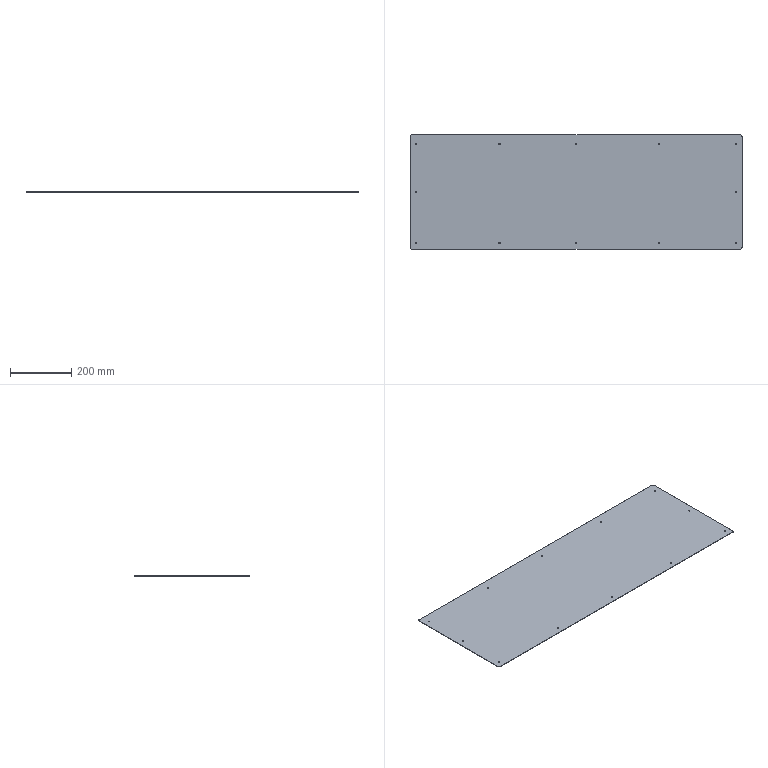Part | SolidWorks | features Fillet 1, FlatPattern 1, ICE 1, SMBaseFlange 1, SheetMetal 1 | 1 solid | 34 faces | box 1087 x 374 x 1.5 mm | volume 609421 mm3 | cylinder 28 | plane 6 | commonest cylinder face diameters 5 x24 10 x4
STEP:
#1=CARTESIAN_POINT('',(-526.,0.,-1.5));
#2=VERTEX_POINT('',#1);
#3=CARTESIAN_POINT('',(-521.,0.,-1.5));
#4=VERTEX_POINT('',#3);
#5=CARTESIAN_POINT('',(-523.5,0.,-1.5));
#6=DIRECTION('',(0.,0.,1.));
#7=DIRECTION('',(1.,0.,0.));
#8=AXIS2_PLACEMENT_3D('',#5,#6,#7);
#9=CIRCLE('',#8,2.5);
#10=EDGE_CURVE('',#2,#4,#9,.T.);
#11=ORIENTED_EDGE('',*,*,#10,.F.);
#12=CARTESIAN_POINT('',(-526.,0.,0.));
#13=VERTEX_POINT('',#12);
#14=CARTESIAN_POINT('',(-526.,0.,-1.5));
#15=DIRECTION('',(0.,0.,1.));
#16=VECTOR('',#15,1000.);
#17=LINE('',#14,#16);
#18=EDGE_CURVE('',#2,#13,#17,.T.);
#19=ORIENTED_EDGE('',*,*,#18,.T.);
#20=CARTESIAN_POINT('',(-521.,0.,0.));
#21=VERTEX_POINT('',#20);
#22=CARTESIAN_POINT('',(-523.5,0.,0.));
#23=DIRECTION('',(0.,0.,1.));
#24=DIRECTION('',(1.,0.,0.));
#25=AXIS2_PLACEMENT_3D('',#22,#23,#24);
#26=CIRCLE('',#25,2.5);
#27=EDGE_CURVE('',#13,#21,#26,.T.);
#28=ORIENTED_EDGE('',*,*,#27,.T.);
#29=CARTESIAN_POINT('',(-521.,0.,-1.5));
#30=DIRECTION('',(0.,0.,1.));
#31=VECTOR('',#30,1000.);
#32=LINE('',#29,#31);
#33=EDGE_CURVE('',#4,#21,#32,.T.);
#34=ORIENTED_EDGE('',*,*,#33,.F.);
#35=EDGE_LOOP('',(#11,#19,#28,#34));
#36=FACE_OUTER_BOUND('',#35,.T.);
#37=CARTESIAN_POINT('',(-523.5,0.,-1.5));
#38=DIRECTION('',(0.,0.,1.));
#39=DIRECTION('',(1.,0.,0.));
#40=AXIS2_PLACEMENT_3D('',#37,#38,#39);
#41=CYLINDRICAL_SURFACE('',#40,2.5);
#42=ADVANCED_FACE('',(#36),#41,.F.);
#43=CARTESIAN_POINT('',(-526.,-167.,-1.5));
#44=VERTEX_POINT('',#43);
#45=CARTESIAN_POINT('',(-521.,-167.,-1.5));
#46=VERTEX_POINT('',#45);
#47=CARTESIAN_POINT('',(-523.5,-167.,-1.5));
#48=DIRECTION('',(0.,0.,1.));
#49=DIRECTION('',(1.,0.,0.));
#50=AXIS2_PLACEMENT_3D('',#47,#48,#49);
#51=CIRCLE('',#50,2.5);
#52=EDGE_CURVE('',#44,#46,#51,.T.);
#53=ORIENTED_EDGE('',*,*,#52,.F.);
#54=CARTESIAN_POINT('',(-526.,-167.,0.));
#55=VERTEX_POINT('',#54);
#56=CARTESIAN_POINT('',(-526.,-167.,-1.5));
#57=DIRECTION('',(0.,0.,1.));
#58=VECTOR('',#57,1000.);
#59=LINE('',#56,#58);
#60=EDGE_CURVE('',#44,#55,#59,.T.);
#61=ORIENTED_EDGE('',*,*,#60,.T.);
#62=CARTESIAN_POINT('',(-521.,-167.,0.));
#63=VERTEX_POINT('',#62);
#64=CARTESIAN_POINT('',(-523.5,-167.,0.));
#65=DIRECTION('',(0.,0.,1.));
#66=DIRECTION('',(1.,0.,0.));
#67=AXIS2_PLACEMENT_3D('',#64,#65,#66);
#68=CIRCLE('',#67,2.5);
#69=EDGE_CURVE('',#55,#63,#68,.T.);
#70=ORIENTED_EDGE('',*,*,#69,.T.);
#71=CARTESIAN_POINT('',(-521.,-167.,-1.5));
#72=DIRECTION('',(0.,0.,1.));
#73=VECTOR('',#72,1000.);
#74=LINE('',#71,#73);
#75=EDGE_CURVE('',#46,#63,#74,.T.);
#76=ORIENTED_EDGE('',*,*,#75,.F.);
#77=EDGE_LOOP('',(#53,#61,#70,#76));
#78=FACE_OUTER_BOUND('',#77,.T.);
#79=CARTESIAN_POINT('',(-523.5,-167.,-1.5));
#80=DIRECTION('',(0.,0.,1.));
#81=DIRECTION('',(1.,0.,0.));
#82=AXIS2_PLACEMENT_3D('',#79,#80,#81);
#83=CYLINDRICAL_SURFACE('',#82,2.5);
#84=ADVANCED_FACE('',(#78),#83,.F.);
#85=CARTESIAN_POINT('',(-253.5,-167.,-1.5));
#86=VERTEX_POINT('',#85);
#87=CARTESIAN_POINT('',(-248.5,-167.,-1.5));
#88=VERTEX_POINT('',#87);
#89=CARTESIAN_POINT('',(-251.,-167.,-1.5));
#90=DIRECTION('',(0.,0.,1.));
#91=DIRECTION('',(1.,0.,0.));
#92=AXIS2_PLACEMENT_3D('',#89,#90,#91);
#93=CIRCLE('',#92,2.5);
#94=EDGE_CURVE('',#86,#88,#93,.T.);
#95=ORIENTED_EDGE('',*,*,#94,.F.);
#96=CARTESIAN_POINT('',(-253.5,-167.,0.));
#97=VERTEX_POINT('',#96);
#98=CARTESIAN_POINT('',(-253.5,-167.,-1.5));
#99=DIRECTION('',(0.,0.,1.));
#100=VECTOR('',#99,1000.);
#101=LINE('',#98,#100);
#102=EDGE_CURVE('',#86,#97,#101,.T.);
#103=ORIENTED_EDGE('',*,*,#102,.T.);
#104=CARTESIAN_POINT('',(-248.5,-167.,0.));
#105=VERTEX_POINT('',#104);
#106=CARTESIAN_POINT('',(-251.,-167.,0.));
#107=DIRECTION('',(0.,0.,1.));
#108=DIRECTION('',(1.,0.,0.));
#109=AXIS2_PLACEMENT_3D('',#106,#107,#108);
#110=CIRCLE('',#109,2.5);
#111=EDGE_CURVE('',#97,#105,#110,.T.);
#112=ORIENTED_EDGE('',*,*,#111,.T.);
#113=CARTESIAN_POINT('',(-248.5,-167.,-1.5));
#114=DIRECTION('',(0.,0.,1.));
#115=VECTOR('',#114,1000.);
#116=LINE('',#113,#115);
#117=EDGE_CURVE('',#88,#105,#116,.T.);
#118=ORIENTED_EDGE('',*,*,#117,.F.);
#119=EDGE_LOOP('',(#95,#103,#112,#118));
#120=FACE_OUTER_BOUND('',#119,.T.);
#121=CARTESIAN_POINT('',(-251.,-167.,-1.5));
#122=DIRECTION('',(0.,0.,1.));
#123=DIRECTION('',(1.,0.,0.));
#124=AXIS2_PLACEMENT_3D('',#121,#122,#123);
#125=CYLINDRICAL_SURFACE('',#124,2.5);
#126=ADVANCED_FACE('',(#120),#125,.F.);
#127=CARTESIAN_POINT('',(-2.5,-167.,-1.5));
#128=VERTEX_POINT('',#127);
#129=CARTESIAN_POINT('',(2.5,-167.,-1.5));
#130=VERTEX_POINT('',#129);
#131=CARTESIAN_POINT('',(0.,-167.,-1.5));
#132=DIRECTION('',(0.,0.,1.));
#133=DIRECTION('',(1.,0.,0.));
#134=AXIS2_PLACEMENT_3D('',#131,#132,#133);
#135=CIRCLE('',#134,2.5);
#136=EDGE_CURVE('',#128,#130,#135,.T.);
#137=ORIENTED_EDGE('',*,*,#136,.F.);
#138=CARTESIAN_POINT('',(-2.5,-167.,0.));
#139=VERTEX_POINT('',#138);
#140=CARTESIAN_POINT('',(-2.5,-167.,-1.5));
#141=DIRECTION('',(0.,0.,1.));
#142=VECTOR('',#141,1000.);
#143=LINE('',#140,#142);
#144=EDGE_CURVE('',#128,#139,#143,.T.);
#145=ORIENTED_EDGE('',*,*,#144,.T.);
#146=CARTESIAN_POINT('',(2.5,-167.,0.));
#147=VERTEX_POINT('',#146);
#148=CARTESIAN_POINT('',(0.,-167.,0.));
#149=DIRECTION('',(0.,0.,1.));
#150=DIRECTION('',(1.,0.,0.));
#151=AXIS2_PLACEMENT_3D('',#148,#149,#150);
#152=CIRCLE('',#151,2.5);
#153=EDGE_CURVE('',#139,#147,#152,.T.);
#154=ORIENTED_EDGE('',*,*,#153,.T.);
#155=CARTESIAN_POINT('',(2.5,-167.,-1.5));
#156=DIRECTION('',(0.,0.,1.));
#157=VECTOR('',#156,1000.);
#158=LINE('',#155,#157);
#159=EDGE_CURVE('',#130,#147,#158,.T.);
#160=ORIENTED_EDGE('',*,*,#159,.F.);
#161=EDGE_LOOP('',(#137,#145,#154,#160));
#162=FACE_OUTER_BOUND('',#161,.T.);
#163=CARTESIAN_POINT('',(0.,-167.,-1.5));
#164=DIRECTION('',(0.,0.,1.));
#165=DIRECTION('',(1.,0.,0.));
#166=AXIS2_PLACEMENT_3D('',#163,#164,#165);
#167=CYLINDRICAL_SURFACE('',#166,2.5);
#168=ADVANCED_FACE('',(#162),#167,.F.);
#169=CARTESIAN_POINT('',(270.,-167.,-1.5));
#170=VERTEX_POINT('',#169);
#171=CARTESIAN_POINT('',(275.,-167.,-1.5));
#172=VERTEX_POINT('',#171);
#173=CARTESIAN_POINT('',(272.5,-167.,-1.5));
#174=DIRECTION('',(0.,0.,1.));
#175=DIRECTION('',(1.,0.,0.));
#176=AXIS2_PLACEMENT_3D('',#173,#174,#175);
#177=CIRCLE('',#176,2.5);
#178=EDGE_CURVE('',#170,#172,#177,.T.);
#179=ORIENTED_EDGE('',*,*,#178,.F.);
#180=CARTESIAN_POINT('',(270.,-167.,0.));
#181=VERTEX_POINT('',#180);
#182=CARTESIAN_POINT('',(270.,-167.,-1.5));
#183=DIRECTION('',(0.,0.,1.));
#184=VECTOR('',#183,1000.);
#185=LINE('',#182,#184);
#186=EDGE_CURVE('',#170,#181,#185,.T.);
#187=ORIENTED_EDGE('',*,*,#186,.T.);
#188=CARTESIAN_POINT('',(275.,-167.,0.));
#189=VERTEX_POINT('',#188);
#190=CARTESIAN_POINT('',(272.5,-167.,0.));
#191=DIRECTION('',(0.,0.,1.));
#192=DIRECTION('',(1.,0.,0.));
#193=AXIS2_PLACEMENT_3D('',#190,#191,#192);
#194=CIRCLE('',#193,2.5);
#195=EDGE_CURVE('',#181,#189,#194,.T.);
#196=ORIENTED_EDGE('',*,*,#195,.T.);
#197=CARTESIAN_POINT('',(275.,-167.,-1.5));
#198=DIRECTION('',(0.,0.,1.));
#199=VECTOR('',#198,1000.);
#200=LINE('',#197,#199);
#201=EDGE_CURVE('',#172,#189,#200,.T.);
#202=ORIENTED_EDGE('',*,*,#201,.F.);
#203=EDGE_LOOP('',(#179,#187,#196,#202));
#204=FACE_OUTER_BOUND('',#203,.T.);
#205=CARTESIAN_POINT('',(272.5,-167.,-1.5));
#206=DIRECTION('',(0.,0.,1.));
#207=DIRECTION('',(1.,0.,0.));
#208=AXIS2_PLACEMENT_3D('',#205,#206,#207);
#209=CYLINDRICAL_SURFACE('',#208,2.5);
#210=ADVANCED_FACE('',(#204),#209,.F.);
#211=CARTESIAN_POINT('',(521.,-167.,-1.5));
#212=VERTEX_POINT('',#211);
#213=CARTESIAN_POINT('',(526.,-167.,-1.5));
#214=VERTEX_POINT('',#213);
#215=CARTESIAN_POINT('',(523.5,-167.,-1.5));
#216=DIRECTION('',(0.,0.,1.));
#217=DIRECTION('',(1.,0.,0.));
#218=AXIS2_PLACEMENT_3D('',#215,#216,#217);
#219=CIRCLE('',#218,2.5);
#220=EDGE_CURVE('',#212,#214,#219,.T.);
#221=ORIENTED_EDGE('',*,*,#220,.F.);
#222=CARTESIAN_POINT('',(521.,-167.,0.));
#223=VERTEX_POINT('',#222);
#224=CARTESIAN_POINT('',(521.,-167.,-1.5));
#225=DIRECTION('',(0.,0.,1.));
#226=VECTOR('',#225,1000.);
#227=LINE('',#224,#226);
#228=EDGE_CURVE('',#212,#223,#227,.T.);
#229=ORIENTED_EDGE('',*,*,#228,.T.);
#230=CARTESIAN_POINT('',(526.,-167.,0.));
#231=VERTEX_POINT('',#230);
#232=CARTESIAN_POINT('',(523.5,-167.,0.));
#233=DIRECTION('',(0.,0.,1.));
#234=DIRECTION('',(1.,0.,0.));
#235=AXIS2_PLACEMENT_3D('',#232,#233,#234);
#236=CIRCLE('',#235,2.5);
#237=EDGE_CURVE('',#223,#231,#236,.T.);
#238=ORIENTED_EDGE('',*,*,#237,.T.);
#239=CARTESIAN_POINT('',(526.,-167.,-1.5));
#240=DIRECTION('',(0.,0.,1.));
#241=VECTOR('',#240,1000.);
#242=LINE('',#239,#241);
#243=EDGE_CURVE('',#214,#231,#242,.T.);
#244=ORIENTED_EDGE('',*,*,#243,.F.);
#245=EDGE_LOOP('',(#221,#229,#238,#244));
#246=FACE_OUTER_BOUND('',#245,.T.);
#247=CARTESIAN_POINT('',(523.5,-167.,-1.5));
#248=DIRECTION('',(0.,0.,1.));
#249=DIRECTION('',(1.,0.,0.));
#250=AXIS2_PLACEMENT_3D('',#247,#248,#249);
#251=CYLINDRICAL_SURFACE('',#250,2.5);
#252=ADVANCED_FACE('',(#246),#251,.F.);
#253=CARTESIAN_POINT('',(521.,0.,-1.5));
#254=VERTEX_POINT('',#253);
#255=CARTESIAN_POINT('',(526.,0.,-1.5));
#256=VERTEX_POINT('',#255);
#257=CARTESIAN_POINT('',(523.5,0.,-1.5));
#258=DIRECTION('',(0.,0.,1.));
#259=DIRECTION('',(1.,0.,0.));
#260=AXIS2_PLACEMENT_3D('',#257,#258,#259);
#261=CIRCLE('',#260,2.5);
#262=EDGE_CURVE('',#254,#256,#261,.T.);
#263=ORIENTED_EDGE('',*,*,#262,.F.);
#264=CARTESIAN_POINT('',(521.,0.,0.));
#265=VERTEX_POINT('',#264);
#266=CARTESIAN_POINT('',(521.,0.,-1.5));
#267=DIRECTION('',(0.,0.,1.));
#268=VECTOR('',#267,1000.);
#269=LINE('',#266,#268);
#270=EDGE_CURVE('',#254,#265,#269,.T.);
#271=ORIENTED_EDGE('',*,*,#270,.T.);
#272=CARTESIAN_POINT('',(526.,0.,0.));
#273=VERTEX_POINT('',#272);
#274=CARTESIAN_POINT('',(523.5,0.,0.));
#275=DIRECTION('',(0.,0.,1.));
#276=DIRECTION('',(1.,0.,0.));
#277=AXIS2_PLACEMENT_3D('',#274,#275,#276);
#278=CIRCLE('',#277,2.5);
#279=EDGE_CURVE('',#265,#273,#278,.T.);
#280=ORIENTED_EDGE('',*,*,#279,.T.);
#281=CARTESIAN_POINT('',(526.,0.,-1.5));
#282=DIRECTION('',(0.,0.,1.));
#283=VECTOR('',#282,1000.);
#284=LINE('',#281,#283);
#285=EDGE_CURVE('',#256,#273,#284,.T.);
#286=ORIENTED_EDGE('',*,*,#285,.F.);
#287=EDGE_LOOP('',(#263,#271,#280,#286));
#288=FACE_OUTER_BOUND('',#287,.T.);
#289=CARTESIAN_POINT('',(523.5,0.,-1.5));
#290=DIRECTION('',(0.,0.,1.));
#291=DIRECTION('',(1.,0.,0.));
#292=AXIS2_PLACEMENT_3D('',#289,#290,#291);
#293=CYLINDRICAL_SURFACE('',#292,2.5);
#294=ADVANCED_FACE('',(#288),#293,.F.);
#295=CARTESIAN_POINT('',(521.,157.,-1.5));
#296=VERTEX_POINT('',#295);
#297=CARTESIAN_POINT('',(526.,157.,-1.5));
#298=VERTEX_POINT('',#297);
#299=CARTESIAN_POINT('',(523.5,157.,-1.5));
#300=DIRECTION('',(0.,0.,1.));
#301=DIRECTION('',(1.,0.,0.));
#302=AXIS2_PLACEMENT_3D('',#299,#300,#301);
#303=CIRCLE('',#302,2.5);
#304=EDGE_CURVE('',#296,#298,#303,.T.);
#305=ORIENTED_EDGE('',*,*,#304,.F.);
#306=CARTESIAN_POINT('',(521.,157.,0.));
#307=VERTEX_POINT('',#306);
#308=CARTESIAN_POINT('',(521.,157.,-1.5));
#309=DIRECTION('',(0.,0.,1.));
#310=VECTOR('',#309,1000.);
#311=LINE('',#308,#310);
#312=EDGE_CURVE('',#296,#307,#311,.T.);
#313=ORIENTED_EDGE('',*,*,#312,.T.);
#314=CARTESIAN_POINT('',(526.,157.,0.));
#315=VERTEX_POINT('',#314);
#316=CARTESIAN_POINT('',(523.5,157.,0.));
#317=DIRECTION('',(0.,0.,1.));
#318=DIRECTION('',(1.,0.,0.));
#319=AXIS2_PLACEMENT_3D('',#316,#317,#318);
#320=CIRCLE('',#319,2.5);
#321=EDGE_CURVE('',#307,#315,#320,.T.);
#322=ORIENTED_EDGE('',*,*,#321,.T.);
#323=CARTESIAN_POINT('',(526.,157.,-1.5));
#324=DIRECTION('',(0.,0.,1.));
#325=VECTOR('',#324,1000.);
#326=LINE('',#323,#325);
#327=EDGE_CURVE('',#298,#315,#326,.T.);
#328=ORIENTED_EDGE('',*,*,#327,.F.);
#329=EDGE_LOOP('',(#305,#313,#322,#328));
#330=FACE_OUTER_BOUND('',#329,.T.);
#331=CARTESIAN_POINT('',(523.5,157.,-1.5));
#332=DIRECTION('',(0.,0.,1.));
#333=DIRECTION('',(1.,0.,0.));
#334=AXIS2_PLACEMENT_3D('',#331,#332,#333);
#335=CYLINDRICAL_SURFACE('',#334,2.5);
#336=ADVANCED_FACE('',(#330),#335,.F.);
#337=CARTESIAN_POINT('',(270.,157.,-1.5));
#338=VERTEX_POINT('',#337);
#339=CARTESIAN_POINT('',(275.,157.,-1.5));
#340=VERTEX_POINT('',#339);
#341=CARTESIAN_POINT('',(272.5,157.,-1.5));
#342=DIRECTION('',(0.,0.,1.));
#343=DIRECTION('',(1.,0.,0.));
#344=AXIS2_PLACEMENT_3D('',#341,#342,#343);
#345=CIRCLE('',#344,2.5);
#346=EDGE_CURVE('',#338,#340,#345,.T.);
#347=ORIENTED_EDGE('',*,*,#346,.F.);
#348=CARTESIAN_POINT('',(270.,157.,0.));
#349=VERTEX_POINT('',#348);
#350=CARTESIAN_POINT('',(270.,157.,-1.5));
#351=DIRECTION('',(0.,0.,1.));
#352=VECTOR('',#351,1000.);
#353=LINE('',#350,#352);
#354=EDGE_CURVE('',#338,#349,#353,.T.);
#355=ORIENTED_EDGE('',*,*,#354,.T.);
#356=CARTESIAN_POINT('',(275.,157.,0.));
#357=VERTEX_POINT('',#356);
#358=CARTESIAN_POINT('',(272.5,157.,0.));
#359=DIRECTION('',(0.,0.,1.));
#360=DIRECTION('',(1.,0.,0.));
#361=AXIS2_PLACEMENT_3D('',#358,#359,#360);
#362=CIRCLE('',#361,2.5);
#363=EDGE_CURVE('',#349,#357,#362,.T.);
#364=ORIENTED_EDGE('',*,*,#363,.T.);
#365=CARTESIAN_POINT('',(275.,157.,-1.5));
#366=DIRECTION('',(0.,0.,1.));
#367=VECTOR('',#366,1000.);
#368=LINE('',#365,#367);
#369=EDGE_CURVE('',#340,#357,#368,.T.);
#370=ORIENTED_EDGE('',*,*,#369,.F.);
#371=EDGE_LOOP('',(#347,#355,#364,#370));
#372=FACE_OUTER_BOUND('',#371,.T.);
#373=CARTESIAN_POINT('',(272.5,157.,-1.5));
#374=DIRECTION('',(0.,0.,1.));
#375=DIRECTION('',(1.,0.,0.));
#376=AXIS2_PLACEMENT_3D('',#373,#374,#375);
#377=CYLINDRICAL_SURFACE('',#376,2.5);
#378=ADVANCED_FACE('',(#372),#377,.F.);
#379=CARTESIAN_POINT('',(-2.5,157.,-1.5));
#380=VERTEX_POINT('',#379);
#381=CARTESIAN_POINT('',(2.5,157.,-1.5));
#382=VERTEX_POINT('',#381);
#383=CARTESIAN_POINT('',(0.,157.,-1.5));
#384=DIRECTION('',(0.,0.,1.));
#385=DIRECTION('',(1.,0.,0.));
#386=AXIS2_PLACEMENT_3D('',#383,#384,#385);
#387=CIRCLE('',#386,2.5);
#388=EDGE_CURVE('',#380,#382,#387,.T.);
#389=ORIENTED_EDGE('',*,*,#388,.F.);
#390=CARTESIAN_POINT('',(-2.5,157.,0.));
#391=VERTEX_POINT('',#390);
#392=CARTESIAN_POINT('',(-2.5,157.,-1.5));
#393=DIRECTION('',(0.,0.,1.));
#394=VECTOR('',#393,1000.);
#395=LINE('',#392,#394);
#396=EDGE_CURVE('',#380,#391,#395,.T.);
#397=ORIENTED_EDGE('',*,*,#396,.T.);
#398=CARTESIAN_POINT('',(2.5,157.,0.));
#399=VERTEX_POINT('',#398);
#400=CARTESIAN_POINT('',(0.,157.,0.));
#401=DIRECTION('',(0.,0.,1.));
#402=DIRECTION('',(1.,0.,0.));
#403=AXIS2_PLACEMENT_3D('',#400,#401,#402);
#404=CIRCLE('',#403,2.5);
#405=EDGE_CURVE('',#391,#399,#404,.T.);
#406=ORIENTED_EDGE('',*,*,#405,.T.);
#407=CARTESIAN_POINT('',(2.5,157.,-1.5));
#408=DIRECTION('',(0.,0.,1.));
#409=VECTOR('',#408,1000.);
#410=LINE('',#407,#409);
#411=EDGE_CURVE('',#382,#399,#410,.T.);
#412=ORIENTED_EDGE('',*,*,#411,.F.);
#413=EDGE_LOOP('',(#389,#397,#406,#412));
#414=FACE_OUTER_BOUND('',#413,.T.);
#415=CARTESIAN_POINT('',(0.,157.,-1.5));
#416=DIRECTION('',(0.,0.,1.));
#417=DIRECTION('',(1.,0.,0.));
#418=AXIS2_PLACEMENT_3D('',#415,#416,#417);
#419=CYLINDRICAL_SURFACE('',#418,2.5);
#420=ADVANCED_FACE('',(#414),#419,.F.);
#421=CARTESIAN_POINT('',(-253.5,157.,-1.5));
#422=VERTEX_POINT('',#421);
#423=CARTESIAN_POINT('',(-248.5,157.,-1.5));
#424=VERTEX_POINT('',#423);
#425=CARTESIAN_POINT('',(-251.,157.,-1.5));
#426=DIRECTION('',(0.,0.,1.));
#427=DIRECTION('',(1.,0.,0.));
#428=AXIS2_PLACEMENT_3D('',#425,#426,#427);
#429=CIRCLE('',#428,2.5);
#430=EDGE_CURVE('',#422,#424,#429,.T.);
#431=ORIENTED_EDGE('',*,*,#430,.F.);
#432=CARTESIAN_POINT('',(-253.5,157.,0.));
#433=VERTEX_POINT('',#432);
#434=CARTESIAN_POINT('',(-253.5,157.,-1.5));
#435=DIRECTION('',(0.,0.,1.));
#436=VECTOR('',#435,1000.);
#437=LINE('',#434,#436);
#438=EDGE_CURVE('',#422,#433,#437,.T.);
#439=ORIENTED_EDGE('',*,*,#438,.T.);
#440=CARTESIAN_POINT('',(-248.5,157.,0.));
#441=VERTEX_POINT('',#440);
#442=CARTESIAN_POINT('',(-251.,157.,0.));
#443=DIRECTION('',(0.,0.,1.));
#444=DIRECTION('',(1.,0.,0.));
#445=AXIS2_PLACEMENT_3D('',#442,#443,#444);
#446=CIRCLE('',#445,2.5);
#447=EDGE_CURVE('',#433,#441,#446,.T.);
#448=ORIENTED_EDGE('',*,*,#447,.T.);
#449=CARTESIAN_POINT('',(-248.5,157.,-1.5));
#450=DIRECTION('',(0.,0.,1.));
#451=VECTOR('',#450,1000.);
#452=LINE('',#449,#451);
#453=EDGE_CURVE('',#424,#441,#452,.T.);
#454=ORIENTED_EDGE('',*,*,#453,.F.);
#455=EDGE_LOOP('',(#431,#439,#448,#454));
#456=FACE_OUTER_BOUND('',#455,.T.);
#457=CARTESIAN_POINT('',(-251.,157.,-1.5));
#458=DIRECTION('',(0.,0.,1.));
#459=DIRECTION('',(1.,0.,0.));
#460=AXIS2_PLACEMENT_3D('',#457,#458,#459);
#461=CYLINDRICAL_SURFACE('',#460,2.5);
#462=ADVANCED_FACE('',(#456),#461,.F.);
#463=CARTESIAN_POINT('',(-526.,157.,-1.5));
#464=VERTEX_POINT('',#463);
#465=CARTESIAN_POINT('',(-521.,157.,-1.5));
#466=VERTEX_POINT('',#465);
#467=CARTESIAN_POINT('',(-523.5,157.,-1.5));
#468=DIRECTION('',(0.,0.,1.));
#469=DIRECTION('',(1.,0.,0.));
#470=AXIS2_PLACEMENT_3D('',#467,#468,#469);
#471=CIRCLE('',#470,2.5);
#472=EDGE_CURVE('',#464,#466,#471,.T.);
#473=ORIENTED_EDGE('',*,*,#472,.F.);
#474=CARTESIAN_POINT('',(-526.,157.,0.));
#475=VERTEX_POINT('',#474);
#476=CARTESIAN_POINT('',(-526.,157.,-1.5));
#477=DIRECTION('',(0.,0.,1.));
#478=VECTOR('',#477,1000.);
#479=LINE('',#476,#478);
#480=EDGE_CURVE('',#464,#475,#479,.T.);
#481=ORIENTED_EDGE('',*,*,#480,.T.);
#482=CARTESIAN_POINT('',(-521.,157.,0.));
#483=VERTEX_POINT('',#482);
#484=CARTESIAN_POINT('',(-523.5,157.,0.));
#485=DIRECTION('',(0.,0.,1.));
#486=DIRECTION('',(1.,0.,0.));
#487=AXIS2_PLACEMENT_3D('',#484,#485,#486);
#488=CIRCLE('',#487,2.5);
#489=EDGE_CURVE('',#475,#483,#488,.T.);
#490=ORIENTED_EDGE('',*,*,#489,.T.);
#491=CARTESIAN_POINT('',(-521.,157.,-1.5));
#492=DIRECTION('',(0.,0.,1.));
#493=VECTOR('',#492,1000.);
#494=LINE('',#491,#493);
#495=EDGE_CURVE('',#466,#483,#494,.T.);
#496=ORIENTED_EDGE('',*,*,#495,.F.);
#497=EDGE_LOOP('',(#473,#481,#490,#496));
#498=FACE_OUTER_BOUND('',#497,.T.);
#499=CARTESIAN_POINT('',(-523.5,157.,-1.5));
#500=DIRECTION('',(0.,0.,1.));
#501=DIRECTION('',(1.,0.,0.));
#502=AXIS2_PLACEMENT_3D('',#499,#500,#501);
#503=CYLINDRICAL_SURFACE('',#502,2.5);
#504=ADVANCED_FACE('',(#498),#503,.F.);
#505=CARTESIAN_POINT('',(543.5,-182.,0.));
#506=VERTEX_POINT('',#505);
#507=CARTESIAN_POINT('',(543.5,182.,0.));
#508=VERTEX_POINT('',#507);
#509=CARTESIAN_POINT('',(543.5,187.,0.));
#510=DIRECTION('',(0.,1.,0.));
#511=VECTOR('',#510,1000.);
#512=LINE('',#509,#511);
#513=EDGE_CURVE('',#506,#508,#512,.T.);
#514=ORIENTED_EDGE('',*,*,#513,.F.);
#515=CARTESIAN_POINT('',(543.5,-182.,-1.5));
#516=VERTEX_POINT('',#515);
#517=CARTESIAN_POINT('',(543.5,-182.,-1.5));
#518=DIRECTION('',(0.,0.,-1.));
#519=VECTOR('',#518,1000.);
#520=LINE('',#517,#519);
#521=EDGE_CURVE('',#506,#516,#520,.T.);
#522=ORIENTED_EDGE('',*,*,#521,.T.);
#523=CARTESIAN_POINT('',(543.5,182.,-1.5));
#524=VERTEX_POINT('',#523);
#525=CARTESIAN_POINT('',(543.5,187.,-1.5));
#526=DIRECTION('',(0.,1.,0.));
#527=VECTOR('',#526,1000.);
#528=LINE('',#525,#527);
#529=EDGE_CURVE('',#516,#524,#528,.T.);
#530=ORIENTED_EDGE('',*,*,#529,.T.);
#531=CARTESIAN_POINT('',(543.5,182.,-1.5));
#532=DIRECTION('',(0.,0.,1.));
#533=VECTOR('',#532,1000.);
#534=LINE('',#531,#533);
#535=EDGE_CURVE('',#524,#508,#534,.T.);
#536=ORIENTED_EDGE('',*,*,#535,.T.);
#537=EDGE_LOOP('',(#514,#522,#530,#536));
#538=FACE_OUTER_BOUND('',#537,.T.);
#539=CARTESIAN_POINT('',(543.5,187.,-1.5));
#540=DIRECTION('',(1.,0.,0.));
#541=DIRECTION('',(0.,0.,-1.));
#542=AXIS2_PLACEMENT_3D('',#539,#540,#541);
#543=PLANE('',#542);
#544=ADVANCED_FACE('',(#538),#543,.T.);
#545=CARTESIAN_POINT('',(-538.5,-187.,0.));
#546=VERTEX_POINT('',#545);
#547=CARTESIAN_POINT('',(538.5,-187.,0.));
#548=VERTEX_POINT('',#547);
#549=CARTESIAN_POINT('',(-543.5,-187.,0.));
#550=DIRECTION('',(1.,0.,0.));
#551=VECTOR('',#550,1000.);
#552=LINE('',#549,#551);
#553=EDGE_CURVE('',#546,#548,#552,.T.);
#554=ORIENTED_EDGE('',*,*,#553,.F.);
#555=CARTESIAN_POINT('',(-538.5,-187.,-1.5));
#556=VERTEX_POINT('',#555);
#557=CARTESIAN_POINT('',(-538.5,-187.,-1.5));
#558=DIRECTION('',(0.,0.,-1.));
#559=VECTOR('',#558,1000.);
#560=LINE('',#557,#559);
#561=EDGE_CURVE('',#546,#556,#560,.T.);
#562=ORIENTED_EDGE('',*,*,#561,.T.);
#563=CARTESIAN_POINT('',(538.5,-187.,-1.5));
#564=VERTEX_POINT('',#563);
#565=CARTESIAN_POINT('',(-543.5,-187.,-1.5));
#566=DIRECTION('',(1.,0.,0.));
#567=VECTOR('',#566,1000.);
#568=LINE('',#565,#567);
#569=EDGE_CURVE('',#556,#564,#568,.T.);
#570=ORIENTED_EDGE('',*,*,#569,.T.);
#571=CARTESIAN_POINT('',(538.5,-187.,-1.5));
#572=DIRECTION('',(0.,0.,1.));
#573=VECTOR('',#572,1000.);
#574=LINE('',#571,#573);
#575=EDGE_CURVE('',#564,#548,#574,.T.);
#576=ORIENTED_EDGE('',*,*,#575,.T.);
#577=EDGE_LOOP('',(#554,#562,#570,#576));
#578=FACE_OUTER_BOUND('',#577,.T.);
#579=CARTESIAN_POINT('',(-543.5,-187.,-1.5));
#580=DIRECTION('',(0.,-1.,0.));
#581=DIRECTION('',(0.,0.,-1.));
#582=AXIS2_PLACEMENT_3D('',#579,#580,#581);
#583=PLANE('',#582);
#584=ADVANCED_FACE('',(#578),#583,.T.);
#585=CARTESIAN_POINT('',(-543.5,182.,-1.5));
#586=VERTEX_POINT('',#585);
#587=CARTESIAN_POINT('',(-543.5,-182.,-1.5));
#588=VERTEX_POINT('',#587);
#589=CARTESIAN_POINT('',(-543.5,187.,-1.5));
#590=DIRECTION('',(0.,-1.,0.));
#591=VECTOR('',#590,1000.);
#592=LINE('',#589,#591);
#593=EDGE_CURVE('',#586,#588,#592,.T.);
#594=ORIENTED_EDGE('',*,*,#593,.T.);
#595=CARTESIAN_POINT('',(-543.5,-182.,0.));
#596=VERTEX_POINT('',#595);
#597=CARTESIAN_POINT('',(-543.5,-182.,-1.5));
#598=DIRECTION('',(0.,0.,1.));
#599=VECTOR('',#598,1000.);
#600=LINE('',#597,#599);
#601=EDGE_CURVE('',#588,#596,#600,.T.);
#602=ORIENTED_EDGE('',*,*,#601,.T.);
#603=CARTESIAN_POINT('',(-543.5,182.,0.));
#604=VERTEX_POINT('',#603);
#605=CARTESIAN_POINT('',(-543.5,187.,0.));
#606=DIRECTION('',(0.,-1.,0.));
#607=VECTOR('',#606,1000.);
#608=LINE('',#605,#607);
#609=EDGE_CURVE('',#604,#596,#608,.T.);
#610=ORIENTED_EDGE('',*,*,#609,.F.);
#611=CARTESIAN_POINT('',(-543.5,182.,-1.5));
#612=DIRECTION('',(0.,0.,-1.));
#613=VECTOR('',#612,1000.);
#614=LINE('',#611,#613);
#615=EDGE_CURVE('',#604,#586,#614,.T.);
#616=ORIENTED_EDGE('',*,*,#615,.T.);
#617=EDGE_LOOP('',(#594,#602,#610,#616));
#618=FACE_OUTER_BOUND('',#617,.T.);
#619=CARTESIAN_POINT('',(-543.5,187.,-1.5));
#620=DIRECTION('',(-1.,0.,0.));
#621=DIRECTION('',(0.,0.,1.));
#622=AXIS2_PLACEMENT_3D('',#619,#620,#621);
#623=PLANE('',#622);
#624=ADVANCED_FACE('',(#618),#623,.T.);
#625=CARTESIAN_POINT('',(538.5,187.,0.));
#626=VERTEX_POINT('',#625);
#627=CARTESIAN_POINT('',(-538.5,187.,0.));
#628=VERTEX_POINT('',#627);
#629=CARTESIAN_POINT('',(-543.5,187.,0.));
#630=DIRECTION('',(-1.,0.,0.));
#631=VECTOR('',#630,1000.);
#632=LINE('',#629,#631);
#633=EDGE_CURVE('',#626,#628,#632,.T.);
#634=ORIENTED_EDGE('',*,*,#633,.F.);
#635=CARTESIAN_POINT('',(538.5,187.,-1.5));
#636=VERTEX_POINT('',#635);
#637=CARTESIAN_POINT('',(538.5,187.,-1.5));
#638=DIRECTION('',(0.,0.,-1.));
#639=VECTOR('',#638,1000.);
#640=LINE('',#637,#639);
#641=EDGE_CURVE('',#626,#636,#640,.T.);
#642=ORIENTED_EDGE('',*,*,#641,.T.);
#643=CARTESIAN_POINT('',(-538.5,187.,-1.5));
#644=VERTEX_POINT('',#643);
#645=CARTESIAN_POINT('',(-543.5,187.,-1.5));
#646=DIRECTION('',(-1.,0.,0.));
#647=VECTOR('',#646,1000.);
#648=LINE('',#645,#647);
#649=EDGE_CURVE('',#636,#644,#648,.T.);
#650=ORIENTED_EDGE('',*,*,#649,.T.);
#651=CARTESIAN_POINT('',(-538.5,187.,-1.5));
#652=DIRECTION('',(0.,0.,1.));
#653=VECTOR('',#652,1000.);
#654=LINE('',#651,#653);
#655=EDGE_CURVE('',#644,#628,#654,.T.);
#656=ORIENTED_EDGE('',*,*,#655,.T.);
#657=EDGE_LOOP('',(#634,#642,#650,#656));
#658=FACE_OUTER_BOUND('',#657,.T.);
#659=CARTESIAN_POINT('',(-543.5,187.,-1.5));
#660=DIRECTION('',(0.,1.,0.));
#661=DIRECTION('',(0.,0.,1.));
#662=AXIS2_PLACEMENT_3D('',#659,#660,#661);
#663=PLANE('',#662);
#664=ADVANCED_FACE('',(#658),#663,.T.);
#665=CARTESIAN_POINT('',(-523.5,0.,-1.5));
#666=DIRECTION('',(0.,0.,1.));
#667=DIRECTION('',(1.,0.,0.));
#668=AXIS2_PLACEMENT_3D('',#665,#666,#667);
#669=CIRCLE('',#668,2.5);
#670=EDGE_CURVE('',#4,#2,#669,.T.);
#671=ORIENTED_EDGE('',*,*,#670,.T.);
#672=ORIENTED_EDGE('',*,*,#10,.T.);
#673=EDGE_LOOP('',(#671,#672));
#674=FACE_BOUND('',#673,.T.);
#675=CARTESIAN_POINT('',(-523.5,-167.,-1.5));
#676=DIRECTION('',(0.,0.,1.));
#677=DIRECTION('',(1.,0.,0.));
#678=AXIS2_PLACEMENT_3D('',#675,#676,#677);
#679=CIRCLE('',#678,2.5);
#680=EDGE_CURVE('',#46,#44,#679,.T.);
#681=ORIENTED_EDGE('',*,*,#680,.T.);
#682=ORIENTED_EDGE('',*,*,#52,.T.);
#683=EDGE_LOOP('',(#681,#682));
#684=FACE_BOUND('',#683,.T.);
#685=CARTESIAN_POINT('',(-251.,-167.,-1.5));
#686=DIRECTION('',(0.,0.,1.));
#687=DIRECTION('',(1.,0.,0.));
#688=AXIS2_PLACEMENT_3D('',#685,#686,#687);
#689=CIRCLE('',#688,2.5);
#690=EDGE_CURVE('',#88,#86,#689,.T.);
#691=ORIENTED_EDGE('',*,*,#690,.T.);
#692=ORIENTED_EDGE('',*,*,#94,.T.);
#693=EDGE_LOOP('',(#691,#692));
#694=FACE_BOUND('',#693,.T.);
#695=CARTESIAN_POINT('',(0.,-167.,-1.5));
#696=DIRECTION('',(0.,0.,1.));
#697=DIRECTION('',(1.,0.,0.));
#698=AXIS2_PLACEMENT_3D('',#695,#696,#697);
#699=CIRCLE('',#698,2.5);
#700=EDGE_CURVE('',#130,#128,#699,.T.);
#701=ORIENTED_EDGE('',*,*,#700,.T.);
#702=ORIENTED_EDGE('',*,*,#136,.T.);
#703=EDGE_LOOP('',(#701,#702));
#704=FACE_BOUND('',#703,.T.);
#705=CARTESIAN_POINT('',(272.5,-167.,-1.5));
#706=DIRECTION('',(0.,0.,1.));
#707=DIRECTION('',(1.,0.,0.));
#708=AXIS2_PLACEMENT_3D('',#705,#706,#707);
#709=CIRCLE('',#708,2.5);
#710=EDGE_CURVE('',#172,#170,#709,.T.);
#711=ORIENTED_EDGE('',*,*,#710,.T.);
#712=ORIENTED_EDGE('',*,*,#178,.T.);
#713=EDGE_LOOP('',(#711,#712));
#714=FACE_BOUND('',#713,.T.);
#715=CARTESIAN_POINT('',(523.5,-167.,-1.5));
#716=DIRECTION('',(0.,0.,1.));
#717=DIRECTION('',(1.,0.,0.));
#718=AXIS2_PLACEMENT_3D('',#715,#716,#717);
#719=CIRCLE('',#718,2.5);
#720=EDGE_CURVE('',#214,#212,#719,.T.);
#721=ORIENTED_EDGE('',*,*,#720,.T.);
#722=ORIENTED_EDGE('',*,*,#220,.T.);
#723=EDGE_LOOP('',(#721,#722));
#724=FACE_BOUND('',#723,.T.);
#725=CARTESIAN_POINT('',(523.5,0.,-1.5));
#726=DIRECTION('',(0.,0.,1.));
#727=DIRECTION('',(1.,0.,0.));
#728=AXIS2_PLACEMENT_3D('',#725,#726,#727);
#729=CIRCLE('',#728,2.5);
#730=EDGE_CURVE('',#256,#254,#729,.T.);
#731=ORIENTED_EDGE('',*,*,#730,.T.);
#732=ORIENTED_EDGE('',*,*,#262,.T.);
#733=EDGE_LOOP('',(#731,#732));
#734=FACE_BOUND('',#733,.T.);
#735=CARTESIAN_POINT('',(523.5,157.,-1.5));
#736=DIRECTION('',(0.,0.,1.));
#737=DIRECTION('',(1.,0.,0.));
#738=AXIS2_PLACEMENT_3D('',#735,#736,#737);
#739=CIRCLE('',#738,2.5);
#740=EDGE_CURVE('',#298,#296,#739,.T.);
#741=ORIENTED_EDGE('',*,*,#740,.T.);
#742=ORIENTED_EDGE('',*,*,#304,.T.);
#743=EDGE_LOOP('',(#741,#742));
#744=FACE_BOUND('',#743,.T.);
#745=CARTESIAN_POINT('',(272.5,157.,-1.5));
#746=DIRECTION('',(0.,0.,1.));
#747=DIRECTION('',(1.,0.,0.));
#748=AXIS2_PLACEMENT_3D('',#745,#746,#747);
#749=CIRCLE('',#748,2.5);
#750=EDGE_CURVE('',#340,#338,#749,.T.);
#751=ORIENTED_EDGE('',*,*,#750,.T.);
#752=ORIENTED_EDGE('',*,*,#346,.T.);
#753=EDGE_LOOP('',(#751,#752));
#754=FACE_BOUND('',#753,.T.);
#755=CARTESIAN_POINT('',(0.,157.,-1.5));
#756=DIRECTION('',(0.,0.,1.));
#757=DIRECTION('',(1.,0.,0.));
#758=AXIS2_PLACEMENT_3D('',#755,#756,#757);
#759=CIRCLE('',#758,2.5);
#760=EDGE_CURVE('',#382,#380,#759,.T.);
#761=ORIENTED_EDGE('',*,*,#760,.T.);
#762=ORIENTED_EDGE('',*,*,#388,.T.);
#763=EDGE_LOOP('',(#761,#762));
#764=FACE_BOUND('',#763,.T.);
#765=CARTESIAN_POINT('',(-251.,157.,-1.5));
#766=DIRECTION('',(0.,0.,1.));
#767=DIRECTION('',(1.,0.,0.));
#768=AXIS2_PLACEMENT_3D('',#765,#766,#767);
#769=CIRCLE('',#768,2.5);
#770=EDGE_CURVE('',#424,#422,#769,.T.);
#771=ORIENTED_EDGE('',*,*,#770,.T.);
#772=ORIENTED_EDGE('',*,*,#430,.T.);
#773=EDGE_LOOP('',(#771,#772));
#774=FACE_BOUND('',#773,.T.);
#775=CARTESIAN_POINT('',(-523.5,157.,-1.5));
#776=DIRECTION('',(0.,0.,1.));
#777=DIRECTION('',(1.,0.,0.));
#778=AXIS2_PLACEMENT_3D('',#775,#776,#777);
#779=CIRCLE('',#778,2.5);
#780=EDGE_CURVE('',#466,#464,#779,.T.);
#781=ORIENTED_EDGE('',*,*,#780,.T.);
#782=ORIENTED_EDGE('',*,*,#472,.T.);
#783=EDGE_LOOP('',(#781,#782));
#784=FACE_BOUND('',#783,.T.);
#785=ORIENTED_EDGE('',*,*,#569,.F.);
#786=CARTESIAN_POINT('',(-538.5,-182.,-1.5));
#787=DIRECTION('',(0.,0.,-1.));
#788=DIRECTION('',(1.,0.,0.));
#789=AXIS2_PLACEMENT_3D('',#786,#787,#788);
#790=CIRCLE('',#789,5.);
#791=EDGE_CURVE('',#556,#588,#790,.T.);
#792=ORIENTED_EDGE('',*,*,#791,.T.);
#793=ORIENTED_EDGE('',*,*,#593,.F.);
#794=CARTESIAN_POINT('',(-538.5,182.,-1.5));
#795=DIRECTION('',(0.,0.,-1.));
#796=DIRECTION('',(1.,0.,0.));
#797=AXIS2_PLACEMENT_3D('',#794,#795,#796);
#798=CIRCLE('',#797,5.);
#799=EDGE_CURVE('',#586,#644,#798,.T.);
#800=ORIENTED_EDGE('',*,*,#799,.T.);
#801=ORIENTED_EDGE('',*,*,#649,.F.);
#802=CARTESIAN_POINT('',(538.5,182.,-1.5));
#803=DIRECTION('',(0.,0.,-1.));
#804=DIRECTION('',(1.,0.,0.));
#805=AXIS2_PLACEMENT_3D('',#802,#803,#804);
#806=CIRCLE('',#805,5.);
#807=EDGE_CURVE('',#636,#524,#806,.T.);
#808=ORIENTED_EDGE('',*,*,#807,.T.);
#809=ORIENTED_EDGE('',*,*,#529,.F.);
#810=CARTESIAN_POINT('',(538.5,-182.,-1.5));
#811=DIRECTION('',(0.,0.,-1.));
#812=DIRECTION('',(1.,0.,0.));
#813=AXIS2_PLACEMENT_3D('',#810,#811,#812);
#814=CIRCLE('',#813,5.);
#815=EDGE_CURVE('',#516,#564,#814,.T.);
#816=ORIENTED_EDGE('',*,*,#815,.T.);
#817=EDGE_LOOP('',(#785,#792,#793,#800,#801,#808,#809,#816));
#818=FACE_OUTER_BOUND('',#817,.T.);
#819=CARTESIAN_POINT('',(0.,0.,-1.5));
#820=DIRECTION('',(0.,0.,1.));
#821=DIRECTION('',(1.,0.,0.));
#822=AXIS2_PLACEMENT_3D('',#819,#820,#821);
#823=PLANE('',#822);
#824=ADVANCED_FACE('',(#674,#684,#694,#704,#714,#724,#734,#744,#754,#764,#774,#784,#818),#823,.F.);
#825=CARTESIAN_POINT('',(-523.5,0.,0.));
#826=DIRECTION('',(0.,0.,1.));
#827=DIRECTION('',(1.,0.,0.));
#828=AXIS2_PLACEMENT_3D('',#825,#826,#827);
#829=CIRCLE('',#828,2.5);
#830=EDGE_CURVE('',#21,#13,#829,.T.);
#831=ORIENTED_EDGE('',*,*,#830,.F.);
#832=ORIENTED_EDGE('',*,*,#27,.F.);
#833=EDGE_LOOP('',(#831,#832));
#834=FACE_BOUND('',#833,.T.);
#835=CARTESIAN_POINT('',(-523.5,-167.,0.));
#836=DIRECTION('',(0.,0.,1.));
#837=DIRECTION('',(1.,0.,0.));
#838=AXIS2_PLACEMENT_3D('',#835,#836,#837);
#839=CIRCLE('',#838,2.5);
#840=EDGE_CURVE('',#63,#55,#839,.T.);
#841=ORIENTED_EDGE('',*,*,#840,.F.);
#842=ORIENTED_EDGE('',*,*,#69,.F.);
#843=EDGE_LOOP('',(#841,#842));
#844=FACE_BOUND('',#843,.T.);
#845=CARTESIAN_POINT('',(-251.,-167.,0.));
#846=DIRECTION('',(0.,0.,1.));
#847=DIRECTION('',(1.,0.,0.));
#848=AXIS2_PLACEMENT_3D('',#845,#846,#847);
#849=CIRCLE('',#848,2.5);
#850=EDGE_CURVE('',#105,#97,#849,.T.);
#851=ORIENTED_EDGE('',*,*,#850,.F.);
#852=ORIENTED_EDGE('',*,*,#111,.F.);
#853=EDGE_LOOP('',(#851,#852));
#854=FACE_BOUND('',#853,.T.);
#855=CARTESIAN_POINT('',(0.,-167.,0.));
#856=DIRECTION('',(0.,0.,1.));
#857=DIRECTION('',(1.,0.,0.));
#858=AXIS2_PLACEMENT_3D('',#855,#856,#857);
#859=CIRCLE('',#858,2.5);
#860=EDGE_CURVE('',#147,#139,#859,.T.);
#861=ORIENTED_EDGE('',*,*,#860,.F.);
#862=ORIENTED_EDGE('',*,*,#153,.F.);
#863=EDGE_LOOP('',(#861,#862));
#864=FACE_BOUND('',#863,.T.);
#865=CARTESIAN_POINT('',(272.5,-167.,0.));
#866=DIRECTION('',(0.,0.,1.));
#867=DIRECTION('',(1.,0.,0.));
#868=AXIS2_PLACEMENT_3D('',#865,#866,#867);
#869=CIRCLE('',#868,2.5);
#870=EDGE_CURVE('',#189,#181,#869,.T.);
#871=ORIENTED_EDGE('',*,*,#870,.F.);
#872=ORIENTED_EDGE('',*,*,#195,.F.);
#873=EDGE_LOOP('',(#871,#872));
#874=FACE_BOUND('',#873,.T.);
#875=CARTESIAN_POINT('',(523.5,-167.,0.));
#876=DIRECTION('',(0.,0.,1.));
#877=DIRECTION('',(1.,0.,0.));
#878=AXIS2_PLACEMENT_3D('',#875,#876,#877);
#879=CIRCLE('',#878,2.5);
#880=EDGE_CURVE('',#231,#223,#879,.T.);
#881=ORIENTED_EDGE('',*,*,#880,.F.);
#882=ORIENTED_EDGE('',*,*,#237,.F.);
#883=EDGE_LOOP('',(#881,#882));
#884=FACE_BOUND('',#883,.T.);
#885=CARTESIAN_POINT('',(523.5,0.,0.));
#886=DIRECTION('',(0.,0.,1.));
#887=DIRECTION('',(1.,0.,0.));
#888=AXIS2_PLACEMENT_3D('',#885,#886,#887);
#889=CIRCLE('',#888,2.5);
#890=EDGE_CURVE('',#273,#265,#889,.T.);
#891=ORIENTED_EDGE('',*,*,#890,.F.);
#892=ORIENTED_EDGE('',*,*,#279,.F.);
#893=EDGE_LOOP('',(#891,#892));
#894=FACE_BOUND('',#893,.T.);
#895=CARTESIAN_POINT('',(523.5,157.,0.));
#896=DIRECTION('',(0.,0.,1.));
#897=DIRECTION('',(1.,0.,0.));
#898=AXIS2_PLACEMENT_3D('',#895,#896,#897);
#899=CIRCLE('',#898,2.5);
#900=EDGE_CURVE('',#315,#307,#899,.T.);
#901=ORIENTED_EDGE('',*,*,#900,.F.);
#902=ORIENTED_EDGE('',*,*,#321,.F.);
#903=EDGE_LOOP('',(#901,#902));
#904=FACE_BOUND('',#903,.T.);
#905=CARTESIAN_POINT('',(272.5,157.,0.));
#906=DIRECTION('',(0.,0.,1.));
#907=DIRECTION('',(1.,0.,0.));
#908=AXIS2_PLACEMENT_3D('',#905,#906,#907);
#909=CIRCLE('',#908,2.5);
#910=EDGE_CURVE('',#357,#349,#909,.T.);
#911=ORIENTED_EDGE('',*,*,#910,.F.);
#912=ORIENTED_EDGE('',*,*,#363,.F.);
#913=EDGE_LOOP('',(#911,#912));
#914=FACE_BOUND('',#913,.T.);
#915=CARTESIAN_POINT('',(0.,157.,0.));
#916=DIRECTION('',(0.,0.,1.));
#917=DIRECTION('',(1.,0.,0.));
#918=AXIS2_PLACEMENT_3D('',#915,#916,#917);
#919=CIRCLE('',#918,2.5);
#920=EDGE_CURVE('',#399,#391,#919,.T.);
#921=ORIENTED_EDGE('',*,*,#920,.F.);
#922=ORIENTED_EDGE('',*,*,#405,.F.);
#923=EDGE_LOOP('',(#921,#922));
#924=FACE_BOUND('',#923,.T.);
#925=CARTESIAN_POINT('',(-251.,157.,0.));
#926=DIRECTION('',(0.,0.,1.));
#927=DIRECTION('',(1.,0.,0.));
#928=AXIS2_PLACEMENT_3D('',#925,#926,#927);
#929=CIRCLE('',#928,2.5);
#930=EDGE_CURVE('',#441,#433,#929,.T.);
#931=ORIENTED_EDGE('',*,*,#930,.F.);
#932=ORIENTED_EDGE('',*,*,#447,.F.);
#933=EDGE_LOOP('',(#931,#932));
#934=FACE_BOUND('',#933,.T.);
#935=CARTESIAN_POINT('',(-523.5,157.,0.));
#936=DIRECTION('',(0.,0.,1.));
#937=DIRECTION('',(1.,0.,0.));
#938=AXIS2_PLACEMENT_3D('',#935,#936,#937);
#939=CIRCLE('',#938,2.5);
#940=EDGE_CURVE('',#483,#475,#939,.T.);
#941=ORIENTED_EDGE('',*,*,#940,.F.);
#942=ORIENTED_EDGE('',*,*,#489,.F.);
#943=EDGE_LOOP('',(#941,#942));
#944=FACE_BOUND('',#943,.T.);
#945=ORIENTED_EDGE('',*,*,#609,.T.);
#946=CARTESIAN_POINT('',(-538.5,-182.,0.));
#947=DIRECTION('',(0.,0.,1.));
#948=DIRECTION('',(1.,0.,0.));
#949=AXIS2_PLACEMENT_3D('',#946,#947,#948);
#950=CIRCLE('',#949,5.);
#951=EDGE_CURVE('',#596,#546,#950,.T.);
#952=ORIENTED_EDGE('',*,*,#951,.T.);
#953=ORIENTED_EDGE('',*,*,#553,.T.);
#954=CARTESIAN_POINT('',(538.5,-182.,0.));
#955=DIRECTION('',(0.,0.,1.));
#956=DIRECTION('',(1.,0.,0.));
#957=AXIS2_PLACEMENT_3D('',#954,#955,#956);
#958=CIRCLE('',#957,5.);
#959=EDGE_CURVE('',#548,#506,#958,.T.);
#960=ORIENTED_EDGE('',*,*,#959,.T.);
#961=ORIENTED_EDGE('',*,*,#513,.T.);
#962=CARTESIAN_POINT('',(538.5,182.,0.));
#963=DIRECTION('',(0.,0.,1.));
#964=DIRECTION('',(1.,0.,0.));
#965=AXIS2_PLACEMENT_3D('',#962,#963,#964);
#966=CIRCLE('',#965,5.);
#967=EDGE_CURVE('',#508,#626,#966,.T.);
#968=ORIENTED_EDGE('',*,*,#967,.T.);
#969=ORIENTED_EDGE('',*,*,#633,.T.);
#970=CARTESIAN_POINT('',(-538.5,182.,0.));
#971=DIRECTION('',(0.,0.,1.));
#972=DIRECTION('',(1.,0.,0.));
#973=AXIS2_PLACEMENT_3D('',#970,#971,#972);
#974=CIRCLE('',#973,5.);
#975=EDGE_CURVE('',#628,#604,#974,.T.);
#976=ORIENTED_EDGE('',*,*,#975,.T.);
#977=EDGE_LOOP('',(#945,#952,#953,#960,#961,#968,#969,#976));
#978=FACE_OUTER_BOUND('',#977,.T.);
#979=CARTESIAN_POINT('',(0.,0.,0.));
#980=DIRECTION('',(0.,0.,1.));
#981=DIRECTION('',(1.,0.,0.));
#982=AXIS2_PLACEMENT_3D('',#979,#980,#981);
#983=PLANE('',#982);
#984=ADVANCED_FACE('',(#834,#844,#854,#864,#874,#884,#894,#904,#914,#924,#934,#944,#978),#983,.T.);
#985=ORIENTED_EDGE('',*,*,#791,.F.);
#986=ORIENTED_EDGE('',*,*,#561,.F.);
#987=ORIENTED_EDGE('',*,*,#951,.F.);
#988=ORIENTED_EDGE('',*,*,#601,.F.);
#989=EDGE_LOOP('',(#985,#986,#987,#988));
#990=FACE_OUTER_BOUND('',#989,.T.);
#991=CARTESIAN_POINT('',(-538.5,-182.,-1.5));
#992=DIRECTION('',(0.,0.,1.));
#993=DIRECTION('',(1.,0.,0.));
#994=AXIS2_PLACEMENT_3D('',#991,#992,#993);
#995=CYLINDRICAL_SURFACE('',#994,5.);
#996=ADVANCED_FACE('',(#990),#995,.T.);
#997=ORIENTED_EDGE('',*,*,#815,.F.);
#998=ORIENTED_EDGE('',*,*,#521,.F.);
#999=ORIENTED_EDGE('',*,*,#959,.F.);
#1000=ORIENTED_EDGE('',*,*,#575,.F.);
#1001=EDGE_LOOP('',(#997,#998,#999,#1000));
#1002=FACE_OUTER_BOUND('',#1001,.T.);
#1003=CARTESIAN_POINT('',(538.5,-182.,-1.5));
#1004=DIRECTION('',(0.,0.,1.));
#1005=DIRECTION('',(1.,0.,0.));
#1006=AXIS2_PLACEMENT_3D('',#1003,#1004,#1005);
#1007=CYLINDRICAL_SURFACE('',#1006,5.);
#1008=ADVANCED_FACE('',(#1002),#1007,.T.);
#1009=ORIENTED_EDGE('',*,*,#807,.F.);
#1010=ORIENTED_EDGE('',*,*,#641,.F.);
#1011=ORIENTED_EDGE('',*,*,#967,.F.);
#1012=ORIENTED_EDGE('',*,*,#535,.F.);
#1013=EDGE_LOOP('',(#1009,#1010,#1011,#1012));
#1014=FACE_OUTER_BOUND('',#1013,.T.);
#1015=CARTESIAN_POINT('',(538.5,182.,-1.5));
#1016=DIRECTION('',(0.,0.,1.));
#1017=DIRECTION('',(1.,0.,0.));
#1018=AXIS2_PLACEMENT_3D('',#1015,#1016,#1017);
#1019=CYLINDRICAL_SURFACE('',#1018,5.);
#1020=ADVANCED_FACE('',(#1014),#1019,.T.);
#1021=ORIENTED_EDGE('',*,*,#799,.F.);
#1022=ORIENTED_EDGE('',*,*,#615,.F.);
#1023=ORIENTED_EDGE('',*,*,#975,.F.);
#1024=ORIENTED_EDGE('',*,*,#655,.F.);
#1025=EDGE_LOOP('',(#1021,#1022,#1023,#1024));
#1026=FACE_OUTER_BOUND('',#1025,.T.);
#1027=CARTESIAN_POINT('',(-538.5,182.,-1.5));
#1028=DIRECTION('',(0.,0.,1.));
#1029=DIRECTION('',(1.,0.,0.));
#1030=AXIS2_PLACEMENT_3D('',#1027,#1028,#1029);
#1031=CYLINDRICAL_SURFACE('',#1030,5.);
#1032=ADVANCED_FACE('',(#1026),#1031,.T.);
#1033=ORIENTED_EDGE('',*,*,#480,.F.);
#1034=ORIENTED_EDGE('',*,*,#780,.F.);
#1035=ORIENTED_EDGE('',*,*,#495,.T.);
#1036=ORIENTED_EDGE('',*,*,#940,.T.);
#1037=EDGE_LOOP('',(#1033,#1034,#1035,#1036));
#1038=FACE_OUTER_BOUND('',#1037,.T.);
#1039=CARTESIAN_POINT('',(-523.5,157.,-1.5));
#1040=DIRECTION('',(0.,0.,1.));
#1041=DIRECTION('',(1.,0.,0.));
#1042=AXIS2_PLACEMENT_3D('',#1039,#1040,#1041);
#1043=CYLINDRICAL_SURFACE('',#1042,2.5);
#1044=ADVANCED_FACE('',(#1038),#1043,.F.);
#1045=ORIENTED_EDGE('',*,*,#438,.F.);
#1046=ORIENTED_EDGE('',*,*,#770,.F.);
#1047=ORIENTED_EDGE('',*,*,#453,.T.);
#1048=ORIENTED_EDGE('',*,*,#930,.T.);
#1049=EDGE_LOOP('',(#1045,#1046,#1047,#1048));
#1050=FACE_OUTER_BOUND('',#1049,.T.);
#1051=CARTESIAN_POINT('',(-251.,157.,-1.5));
#1052=DIRECTION('',(0.,0.,1.));
#1053=DIRECTION('',(1.,0.,0.));
#1054=AXIS2_PLACEMENT_3D('',#1051,#1052,#1053);
#1055=CYLINDRICAL_SURFACE('',#1054,2.5);
#1056=ADVANCED_FACE('',(#1050),#1055,.F.);
#1057=ORIENTED_EDGE('',*,*,#396,.F.);
#1058=ORIENTED_EDGE('',*,*,#760,.F.);
#1059=ORIENTED_EDGE('',*,*,#411,.T.);
#1060=ORIENTED_EDGE('',*,*,#920,.T.);
#1061=EDGE_LOOP('',(#1057,#1058,#1059,#1060));
#1062=FACE_OUTER_BOUND('',#1061,.T.);
#1063=CARTESIAN_POINT('',(0.,157.,-1.5));
#1064=DIRECTION('',(0.,0.,1.));
#1065=DIRECTION('',(1.,0.,0.));
#1066=AXIS2_PLACEMENT_3D('',#1063,#1064,#1065);
#1067=CYLINDRICAL_SURFACE('',#1066,2.5);
#1068=ADVANCED_FACE('',(#1062),#1067,.F.);
#1069=ORIENTED_EDGE('',*,*,#354,.F.);
#1070=ORIENTED_EDGE('',*,*,#750,.F.);
#1071=ORIENTED_EDGE('',*,*,#369,.T.);
#1072=ORIENTED_EDGE('',*,*,#910,.T.);
#1073=EDGE_LOOP('',(#1069,#1070,#1071,#1072));
#1074=FACE_OUTER_BOUND('',#1073,.T.);
#1075=CARTESIAN_POINT('',(272.5,157.,-1.5));
#1076=DIRECTION('',(0.,0.,1.));
#1077=DIRECTION('',(1.,0.,0.));
#1078=AXIS2_PLACEMENT_3D('',#1075,#1076,#1077);
#1079=CYLINDRICAL_SURFACE('',#1078,2.5);
#1080=ADVANCED_FACE('',(#1074),#1079,.F.);
#1081=ORIENTED_EDGE('',*,*,#312,.F.);
#1082=ORIENTED_EDGE('',*,*,#740,.F.);
#1083=ORIENTED_EDGE('',*,*,#327,.T.);
#1084=ORIENTED_EDGE('',*,*,#900,.T.);
#1085=EDGE_LOOP('',(#1081,#1082,#1083,#1084));
#1086=FACE_OUTER_BOUND('',#1085,.T.);
#1087=CARTESIAN_POINT('',(523.5,157.,-1.5));
#1088=DIRECTION('',(0.,0.,1.));
#1089=DIRECTION('',(1.,0.,0.));
#1090=AXIS2_PLACEMENT_3D('',#1087,#1088,#1089);
#1091=CYLINDRICAL_SURFACE('',#1090,2.5);
#1092=ADVANCED_FACE('',(#1086),#1091,.F.);
#1093=ORIENTED_EDGE('',*,*,#270,.F.);
#1094=ORIENTED_EDGE('',*,*,#730,.F.);
#1095=ORIENTED_EDGE('',*,*,#285,.T.);
#1096=ORIENTED_EDGE('',*,*,#890,.T.);
#1097=EDGE_LOOP('',(#1093,#1094,#1095,#1096));
#1098=FACE_OUTER_BOUND('',#1097,.T.);
#1099=CARTESIAN_POINT('',(523.5,0.,-1.5));
#1100=DIRECTION('',(0.,0.,1.));
#1101=DIRECTION('',(1.,0.,0.));
#1102=AXIS2_PLACEMENT_3D('',#1099,#1100,#1101);
#1103=CYLINDRICAL_SURFACE('',#1102,2.5);
#1104=ADVANCED_FACE('',(#1098),#1103,.F.);
#1105=ORIENTED_EDGE('',*,*,#228,.F.);
#1106=ORIENTED_EDGE('',*,*,#720,.F.);
#1107=ORIENTED_EDGE('',*,*,#243,.T.);
#1108=ORIENTED_EDGE('',*,*,#880,.T.);
#1109=EDGE_LOOP('',(#1105,#1106,#1107,#1108));
#1110=FACE_OUTER_BOUND('',#1109,.T.);
#1111=CARTESIAN_POINT('',(523.5,-167.,-1.5));
#1112=DIRECTION('',(0.,0.,1.));
#1113=DIRECTION('',(1.,0.,0.));
#1114=AXIS2_PLACEMENT_3D('',#1111,#1112,#1113);
#1115=CYLINDRICAL_SURFACE('',#1114,2.5);
#1116=ADVANCED_FACE('',(#1110),#1115,.F.);
#1117=ORIENTED_EDGE('',*,*,#186,.F.);
#1118=ORIENTED_EDGE('',*,*,#710,.F.);
#1119=ORIENTED_EDGE('',*,*,#201,.T.);
#1120=ORIENTED_EDGE('',*,*,#870,.T.);
#1121=EDGE_LOOP('',(#1117,#1118,#1119,#1120));
#1122=FACE_OUTER_BOUND('',#1121,.T.);
#1123=CARTESIAN_POINT('',(272.5,-167.,-1.5));
#1124=DIRECTION('',(0.,0.,1.));
#1125=DIRECTION('',(1.,0.,0.));
#1126=AXIS2_PLACEMENT_3D('',#1123,#1124,#1125);
#1127=CYLINDRICAL_SURFACE('',#1126,2.5);
#1128=ADVANCED_FACE('',(#1122),#1127,.F.);
#1129=ORIENTED_EDGE('',*,*,#144,.F.);
#1130=ORIENTED_EDGE('',*,*,#700,.F.);
#1131=ORIENTED_EDGE('',*,*,#159,.T.);
#1132=ORIENTED_EDGE('',*,*,#860,.T.);
#1133=EDGE_LOOP('',(#1129,#1130,#1131,#1132));
#1134=FACE_OUTER_BOUND('',#1133,.T.);
#1135=CARTESIAN_POINT('',(0.,-167.,-1.5));
#1136=DIRECTION('',(0.,0.,1.));
#1137=DIRECTION('',(1.,0.,0.));
#1138=AXIS2_PLACEMENT_3D('',#1135,#1136,#1137);
#1139=CYLINDRICAL_SURFACE('',#1138,2.5);
#1140=ADVANCED_FACE('',(#1134),#1139,.F.);
#1141=ORIENTED_EDGE('',*,*,#102,.F.);
#1142=ORIENTED_EDGE('',*,*,#690,.F.);
#1143=ORIENTED_EDGE('',*,*,#117,.T.);
#1144=ORIENTED_EDGE('',*,*,#850,.T.);
#1145=EDGE_LOOP('',(#1141,#1142,#1143,#1144));
#1146=FACE_OUTER_BOUND('',#1145,.T.);
#1147=CARTESIAN_POINT('',(-251.,-167.,-1.5));
#1148=DIRECTION('',(0.,0.,1.));
#1149=DIRECTION('',(1.,0.,0.));
#1150=AXIS2_PLACEMENT_3D('',#1147,#1148,#1149);
#1151=CYLINDRICAL_SURFACE('',#1150,2.5);
#1152=ADVANCED_FACE('',(#1146),#1151,.F.);
#1153=ORIENTED_EDGE('',*,*,#60,.F.);
#1154=ORIENTED_EDGE('',*,*,#680,.F.);
#1155=ORIENTED_EDGE('',*,*,#75,.T.);
#1156=ORIENTED_EDGE('',*,*,#840,.T.);
#1157=EDGE_LOOP('',(#1153,#1154,#1155,#1156));
#1158=FACE_OUTER_BOUND('',#1157,.T.);
#1159=CARTESIAN_POINT('',(-523.5,-167.,-1.5));
#1160=DIRECTION('',(0.,0.,1.));
#1161=DIRECTION('',(1.,0.,0.));
#1162=AXIS2_PLACEMENT_3D('',#1159,#1160,#1161);
#1163=CYLINDRICAL_SURFACE('',#1162,2.5);
#1164=ADVANCED_FACE('',(#1158),#1163,.F.);
#1165=ORIENTED_EDGE('',*,*,#18,.F.);
#1166=ORIENTED_EDGE('',*,*,#670,.F.);
#1167=ORIENTED_EDGE('',*,*,#33,.T.);
#1168=ORIENTED_EDGE('',*,*,#830,.T.);
#1169=EDGE_LOOP('',(#1165,#1166,#1167,#1168));
#1170=FACE_OUTER_BOUND('',#1169,.T.);
#1171=CARTESIAN_POINT('',(-523.5,0.,-1.5));
#1172=DIRECTION('',(0.,0.,1.));
#1173=DIRECTION('',(1.,0.,0.));
#1174=AXIS2_PLACEMENT_3D('',#1171,#1172,#1173);
#1175=CYLINDRICAL_SURFACE('',#1174,2.5);
#1176=ADVANCED_FACE('',(#1170),#1175,.F.);
#1177=CLOSED_SHELL('',(#42,#84,#126,#168,#210,#252,#294,#336,#378,#420,#462,#504,#544,#584,#624,#664,#824,#984,#996,#1008,#1020,#1032,#1044,#1056,#1068,#1080,#1092,#1104,#1116,#1128,#1140,#1152,#1164,#1176));
#1178=MANIFOLD_SOLID_BREP('',#1177);
#1179=CARTESIAN_POINT('',(0.,0.,0.));
#1180=DIRECTION('',(0.,0.,1.));
#1181=DIRECTION('',(1.,0.,0.));
#1182=AXIS2_PLACEMENT_3D('',#1179,#1180,#1181);
#1183=(LENGTH_UNIT()NAMED_UNIT(*)SI_UNIT(.MILLI.,.METRE.));
#1184=UNCERTAINTY_MEASURE_WITH_UNIT(LENGTH_MEASURE(0.00001),#1183,'','');
#1185=(NAMED_UNIT(*)PLANE_ANGLE_UNIT()SI_UNIT($,.RADIAN.));
#1186=(NAMED_UNIT(*)SI_UNIT($,.STERADIAN.)SOLID_ANGLE_UNIT());
#1187=(GEOMETRIC_REPRESENTATION_CONTEXT(3)GLOBAL_UNCERTAINTY_ASSIGNED_CONTEXT((#1184))GLOBAL_UNIT_ASSIGNED_CONTEXT((#1183,#1185,#1186))REPRESENTATION_CONTEXT('',''));
#1188=ADVANCED_BREP_SHAPE_REPRESENTATION('',(#1178,#1182),#1187);